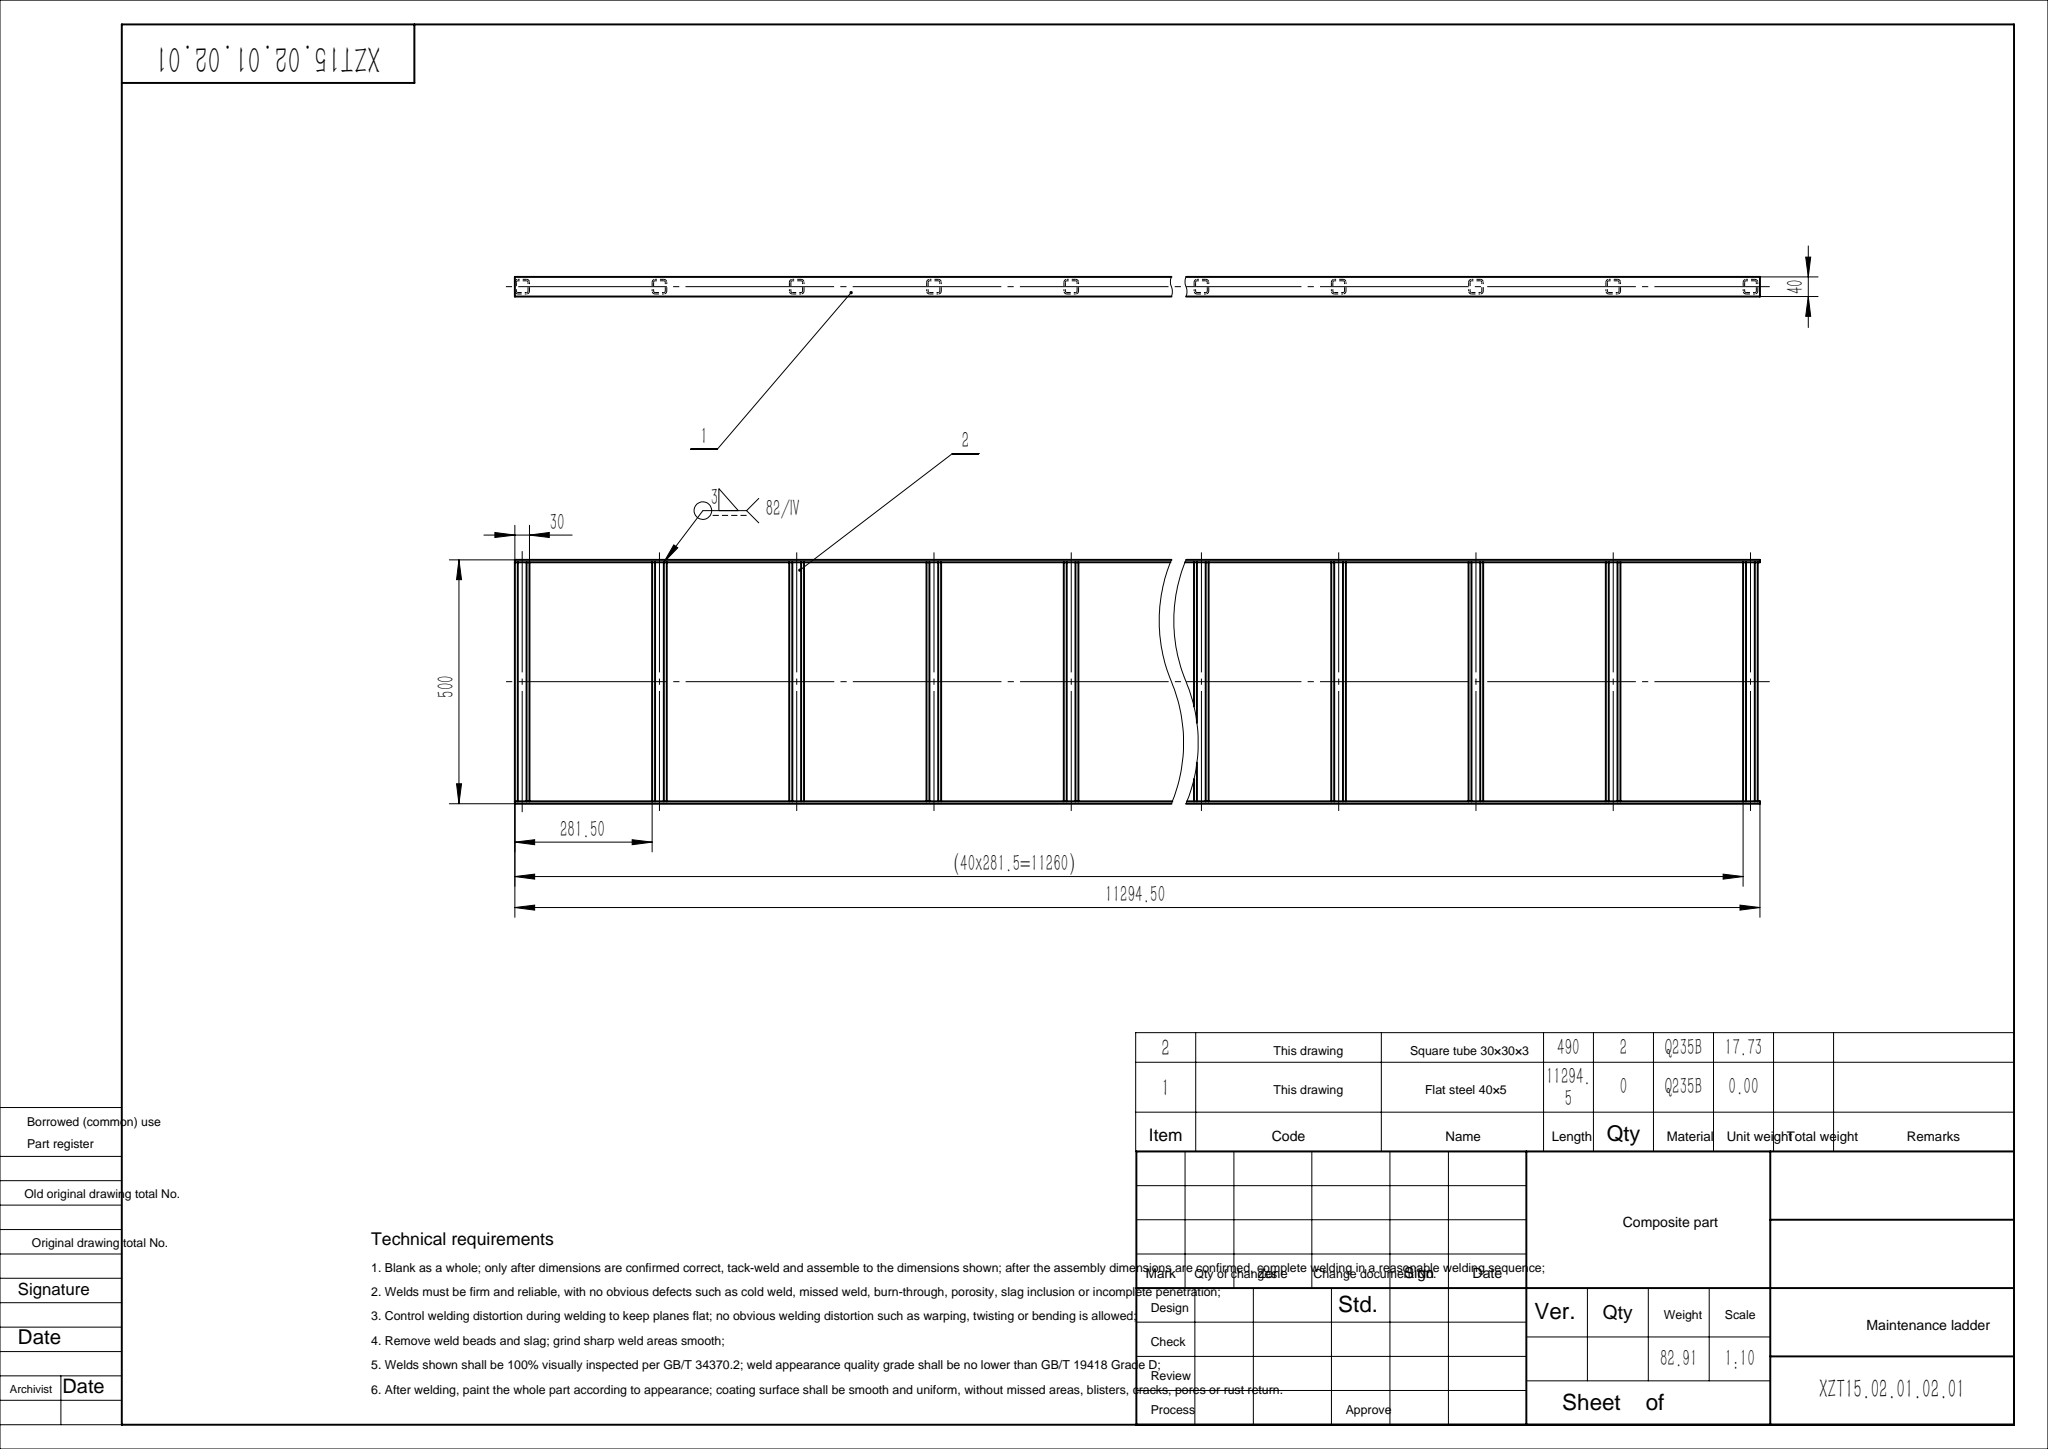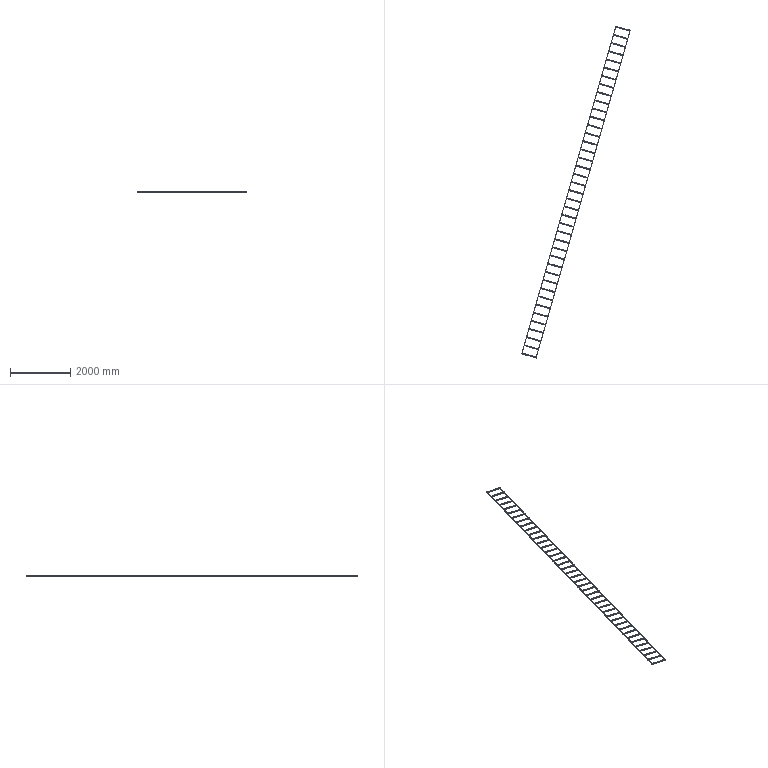Part | SolidWorks | features WeldMemberFeat 2, Chamfer 1, ICE 1, LPattern 1, Sweep 1, WeldCornerFeat 1, WeldmentFeature 1 | 43 solids | 750 faces | box 3594 x 10995 x 40 mm | volume 10561334 mm3 | plane 422 | cylinder 328 | commonest cylinder face diameters 6 x164 12 x164